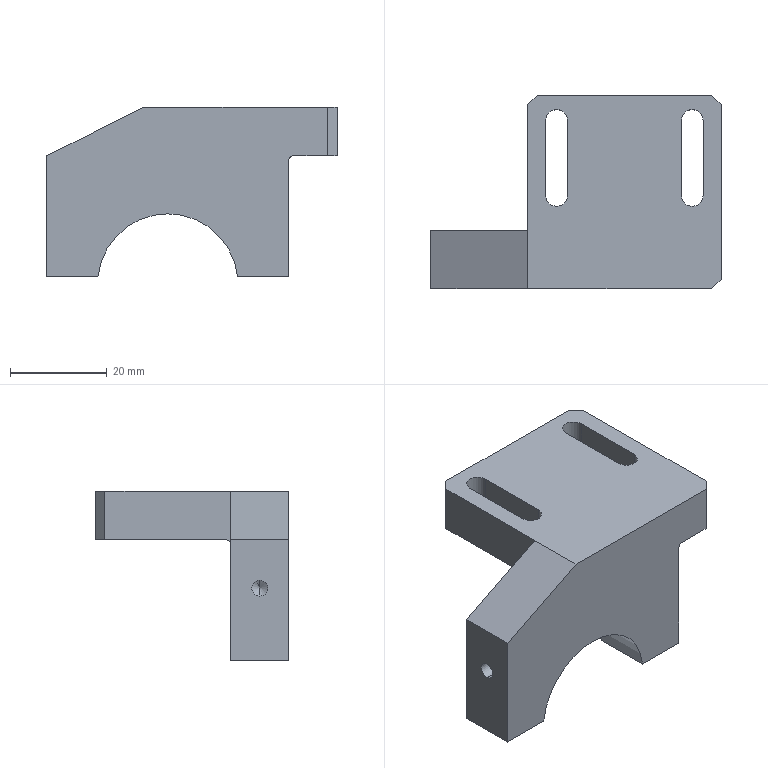NC program | NX | posted with a generic post | part box 60 x 40 x 35 mm
Whole program:
N10 G17 G21 G94 G90
(FLOOR_WALL_COPY , TOOL : D80)
N12 T19 M6
N14 G54
N16 G17 G0 G90 X73. Y0. S6500 M3
N18 G43 Z30. H19
N20 Z7.
N22 G94 G1 Z4. F1500.
N24 X70.
N26 X-70.
N28 X-73.
N30 Z7.
N32 G0 Z30.
N34 X73.
N36 Z6.
N38 G1 Z3.
N40 X70.
N42 X-70.
N44 X-73.
N46 Z6.
N48 G0 Z30.
N50 X73.
N52 Z5.
N54 G1 Z2.
N56 X70.
N58 X-70.
N60 X-73.
N62 Z5.
N64 G0 Z30.
N66 X73.
N68 Z4.
N70 G1 Z1.
N72 X70.
N74 X-70.
N76 X-73.
N78 Z4.
N80 G0 Z30.
N82 X73.
N84 Z3.
N86 G1 Z0.
N88 X70.
N90 X-70.
N92 X-73.
N94 Z3.
N96 G0 Z30.
N98 M5
(PLANAR_MILL_COPY_COPY_COPY_COPY_COPY , TOOL : D6A45)
N100 T01 M6
N102 G54
N104 G17 G0 G90 X12.17 Y5.3 S9500 M3
N106 G43 Z30. H1
N108 Z0.5
N110 G94 G1 Z-1. F1250.
N112 X11.766 Y6.
N114 G3 X10.9 Y6.5 R1.
N116 G1 Y-17.959
N118 G2 X10.607 Y-18.666 R1.
N120 G1 X8.666 Y-20.607
N122 G2 X7.959 Y-20.9 R1.
N124 G1 X-27.959
N126 G2 X-28.666 Y-20.607 R1.
N128 G1 X-30.607 Y-18.666
N130 G2 X-30.9 Y-17.959 R1.
N132 G1 Y17.959
N134 G2 X-30.607 Y18.666 R1.
N136 G1 X-28.666 Y20.607
N138 G2 X-27.959 Y20.9 R1.
N140 G1 X8.8
N142 G3 X8.92 Y21.893 R1.
N144 G1 X8.714 Y22.374
N146 Z0.5
N148 G0 Z30.
N150 X4.15 Y-8.27
N152 Z0.5
N154 G1 Z-1.
N156 X4.85 Y-7.866
N158 G3 X5.35 Y-7. R1.
N160 G1 Y0.75
N162 G3 X4. Y2.1 R1.35
N164 X2.65 Y0.75 R1.35
N166 G1 Y-14.75
N168 G3 X4. Y-16.1 R1.35
N170 X5.35 Y-14.75 R1.35
N172 G1 Y-7.
N174 G3 X4.85 Y-6.134 R1.
N176 G1 X4.15 Y-5.73
N178 Z0.5
N180 G0 Z30.
N182 X-24.15
N184 Z0.5
N186 G1 Z-1.
N188 X-24.85 Y-6.134
N190 G3 X-25.35 Y-7. R1.
N192 G1 Y-14.75
N194 G3 X-24. Y-16.1 R1.35
N196 X-22.65 Y-14.75 R1.35
N198 G1 Y0.75
N200 G3 X-24. Y2.1 R1.35
N202 X-25.35 Y0.75 R1.35
N204 G1 Y-7.
N206 G3 X-24.85 Y-7.866 R1.
N208 G1 X-24.15 Y-8.27
N210 Z0.5
N212 G0 Z30.
N214 M5
N216 M2